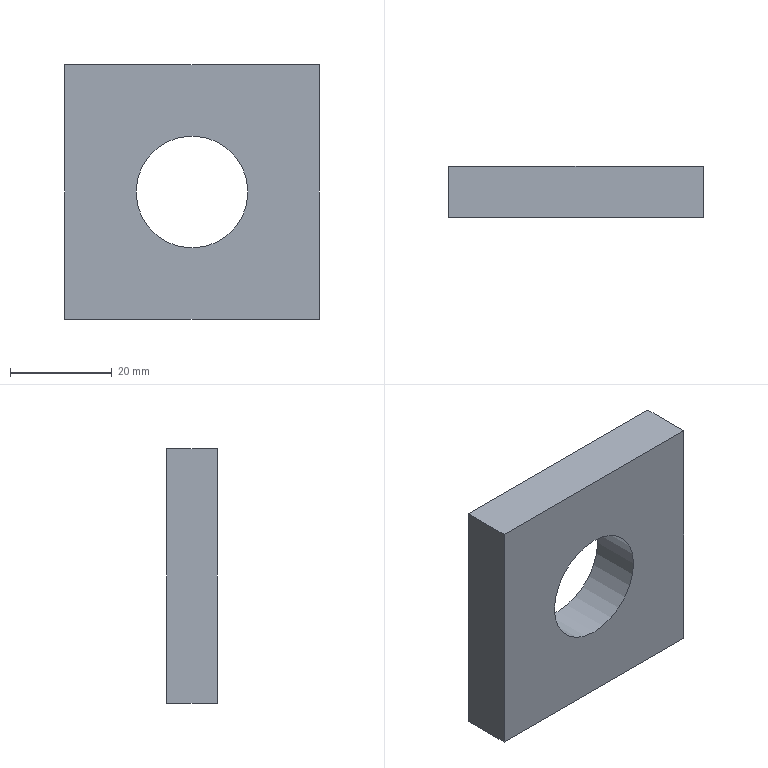Part | STEP file | PN_0016 anchor bolt shim_Default<As Machined> | 1 solid | 7 faces | box 50 x 10 x 50 mm | volume 21199 mm3 | plane 6 | cylinder 1 | commonest cylinder face diameters 22 x1
STEP:
#1=CARTESIAN_POINT('',(0.,0.,0.));
#2=DIRECTION('',(0.,0.,1.));
#3=DIRECTION('',(1.,0.,0.));
#4=AXIS2_PLACEMENT_3D('',#1,#2,#3);
#5=CARTESIAN_POINT('',(25.,10.,25.));
#6=VERTEX_POINT('',#5);
#7=CARTESIAN_POINT('',(25.,10.,-25.));
#8=VERTEX_POINT('',#7);
#9=CARTESIAN_POINT('',(25.,10.,25.));
#10=DIRECTION('',(0.,0.,-1.));
#11=VECTOR('',#10,1.);
#12=LINE('',#9,#11);
#13=CARTESIAN_POINT('',(0.,10.,0.));
#14=DIRECTION('',(0.,-1.,0.));
#15=DIRECTION('',(0.,0.,-1.));
#16=AXIS2_PLACEMENT_3D('',#13,#14,#15);
#17=PLANE('',#16);
#18=CARTESIAN_POINT('',(-25.,25.));
#19=DIRECTION('',(1.,0.));
#20=VECTOR('',#19,1.);
#21=LINE('',#18,#20);
#22=(GEOMETRIC_REPRESENTATION_CONTEXT(2)PARAMETRIC_REPRESENTATION_CONTEXT()REPRESENTATION_CONTEXT('',''));
#23=DEFINITIONAL_REPRESENTATION('',(#21),#22);
#24=PCURVE('',#17,#23);
#25=CARTESIAN_POINT('',(25.,10.,25.));
#26=DIRECTION('',(-1.,0.,0.));
#27=DIRECTION('',(0.,0.,1.));
#28=AXIS2_PLACEMENT_3D('',#25,#26,#27);
#29=PLANE('',#28);
#30=CARTESIAN_POINT('',(0.,0.));
#31=DIRECTION('',(-1.,0.));
#32=VECTOR('',#31,1.);
#33=LINE('',#30,#32);
#34=(GEOMETRIC_REPRESENTATION_CONTEXT(2)PARAMETRIC_REPRESENTATION_CONTEXT()REPRESENTATION_CONTEXT('',''));
#35=DEFINITIONAL_REPRESENTATION('',(#33),#34);
#36=PCURVE('',#29,#35);
#37=SURFACE_CURVE('',#12,(#24,#36),.PCURVE_S1.);
#38=EDGE_CURVE('',#6,#8,#37,.T.);
#39=ORIENTED_EDGE('',*,*,#38,.T.);
#40=CARTESIAN_POINT('',(-25.,10.,-25.));
#41=VERTEX_POINT('',#40);
#42=CARTESIAN_POINT('',(-25.,10.,-25.));
#43=DIRECTION('',(-1.,0.,0.));
#44=VECTOR('',#43,1.);
#45=LINE('',#42,#44);
#46=CARTESIAN_POINT('',(25.,-25.));
#47=DIRECTION('',(0.,-1.));
#48=VECTOR('',#47,1.);
#49=LINE('',#46,#48);
#50=(GEOMETRIC_REPRESENTATION_CONTEXT(2)PARAMETRIC_REPRESENTATION_CONTEXT()REPRESENTATION_CONTEXT('',''));
#51=DEFINITIONAL_REPRESENTATION('',(#49),#50);
#52=PCURVE('',#17,#51);
#53=CARTESIAN_POINT('',(-25.,10.,-25.));
#54=DIRECTION('',(0.,0.,1.));
#55=DIRECTION('',(1.,0.,0.));
#56=AXIS2_PLACEMENT_3D('',#53,#54,#55);
#57=PLANE('',#56);
#58=CARTESIAN_POINT('',(0.,0.));
#59=DIRECTION('',(-1.,0.));
#60=VECTOR('',#59,1.);
#61=LINE('',#58,#60);
#62=(GEOMETRIC_REPRESENTATION_CONTEXT(2)PARAMETRIC_REPRESENTATION_CONTEXT()REPRESENTATION_CONTEXT('',''));
#63=DEFINITIONAL_REPRESENTATION('',(#61),#62);
#64=PCURVE('',#57,#63);
#65=SURFACE_CURVE('',#45,(#52,#64),.PCURVE_S1.);
#66=EDGE_CURVE('',#8,#41,#65,.T.);
#67=ORIENTED_EDGE('',*,*,#66,.T.);
#68=CARTESIAN_POINT('',(-25.,10.,25.));
#69=VERTEX_POINT('',#68);
#70=CARTESIAN_POINT('',(-25.,10.,25.));
#71=DIRECTION('',(0.,0.,1.));
#72=VECTOR('',#71,1.);
#73=LINE('',#70,#72);
#74=CARTESIAN_POINT('',(-25.,-25.));
#75=DIRECTION('',(-1.,0.));
#76=VECTOR('',#75,1.);
#77=LINE('',#74,#76);
#78=(GEOMETRIC_REPRESENTATION_CONTEXT(2)PARAMETRIC_REPRESENTATION_CONTEXT()REPRESENTATION_CONTEXT('',''));
#79=DEFINITIONAL_REPRESENTATION('',(#77),#78);
#80=PCURVE('',#17,#79);
#81=CARTESIAN_POINT('',(-25.,10.,25.));
#82=DIRECTION('',(1.,0.,0.));
#83=DIRECTION('',(0.,0.,-1.));
#84=AXIS2_PLACEMENT_3D('',#81,#82,#83);
#85=PLANE('',#84);
#86=CARTESIAN_POINT('',(0.,0.));
#87=DIRECTION('',(-1.,0.));
#88=VECTOR('',#87,1.);
#89=LINE('',#86,#88);
#90=(GEOMETRIC_REPRESENTATION_CONTEXT(2)PARAMETRIC_REPRESENTATION_CONTEXT()REPRESENTATION_CONTEXT('',''));
#91=DEFINITIONAL_REPRESENTATION('',(#89),#90);
#92=PCURVE('',#85,#91);
#93=SURFACE_CURVE('',#73,(#80,#92),.PCURVE_S1.);
#94=EDGE_CURVE('',#41,#69,#93,.T.);
#95=ORIENTED_EDGE('',*,*,#94,.T.);
#96=CARTESIAN_POINT('',(-25.,10.,25.));
#97=DIRECTION('',(1.,0.,0.));
#98=VECTOR('',#97,1.);
#99=LINE('',#96,#98);
#100=CARTESIAN_POINT('',(-25.,-25.));
#101=DIRECTION('',(0.,1.));
#102=VECTOR('',#101,1.);
#103=LINE('',#100,#102);
#104=(GEOMETRIC_REPRESENTATION_CONTEXT(2)PARAMETRIC_REPRESENTATION_CONTEXT()REPRESENTATION_CONTEXT('',''));
#105=DEFINITIONAL_REPRESENTATION('',(#103),#104);
#106=PCURVE('',#17,#105);
#107=CARTESIAN_POINT('',(-25.,10.,25.));
#108=DIRECTION('',(0.,0.,-1.));
#109=DIRECTION('',(-1.,0.,0.));
#110=AXIS2_PLACEMENT_3D('',#107,#108,#109);
#111=PLANE('',#110);
#112=CARTESIAN_POINT('',(0.,0.));
#113=DIRECTION('',(-1.,0.));
#114=VECTOR('',#113,1.);
#115=LINE('',#112,#114);
#116=(GEOMETRIC_REPRESENTATION_CONTEXT(2)PARAMETRIC_REPRESENTATION_CONTEXT()REPRESENTATION_CONTEXT('',''));
#117=DEFINITIONAL_REPRESENTATION('',(#115),#116);
#118=PCURVE('',#111,#117);
#119=SURFACE_CURVE('',#99,(#106,#118),.PCURVE_S1.);
#120=EDGE_CURVE('',#69,#6,#119,.T.);
#121=ORIENTED_EDGE('',*,*,#120,.T.);
#122=EDGE_LOOP('',(#39,#67,#95,#121));
#123=FACE_BOUND('',#122,.T.);
#124=CARTESIAN_POINT('',(0.,10.,11.));
#125=VERTEX_POINT('',#124);
#126=CARTESIAN_POINT('',(0.,10.,0.));
#127=DIRECTION('',(0.,1.,0.));
#128=DIRECTION('',(0.,0.,1.));
#129=AXIS2_PLACEMENT_3D('',#126,#127,#128);
#130=CIRCLE('',#129,11.);
#131=CARTESIAN_POINT('',(-11.,0.));
#132=CARTESIAN_POINT('',(-11.,19.053));
#133=CARTESIAN_POINT('',(5.5,9.526));
#134=CARTESIAN_POINT('',(22.,0.));
#135=CARTESIAN_POINT('',(5.5,-9.526));
#136=CARTESIAN_POINT('',(-11.,-19.053));
#137=CARTESIAN_POINT('',(-11.,0.));
#138=(BOUNDED_CURVE()B_SPLINE_CURVE(2,(#131,#132,#133,#134,#135,#136,#137),.UNSPECIFIED.,.T.,.F.)B_SPLINE_CURVE_WITH_KNOTS((1,2,2,2,2,1),(-2.094,0.,2.094,4.189,6.283,8.378),.UNSPECIFIED.)CURVE()GEOMETRIC_REPRESENTATION_ITEM()RATIONAL_B_SPLINE_CURVE((1.,0.5,1.,0.5,1.,0.5,1.))REPRESENTATION_ITEM(''));
#139=(GEOMETRIC_REPRESENTATION_CONTEXT(2)PARAMETRIC_REPRESENTATION_CONTEXT()REPRESENTATION_CONTEXT('',''));
#140=DEFINITIONAL_REPRESENTATION('',(#138),#139);
#141=PCURVE('',#17,#140);
#142=CARTESIAN_POINT('',(0.,10.,0.));
#143=DIRECTION('',(0.,-1.,0.));
#144=DIRECTION('',(0.,0.,-1.));
#145=AXIS2_PLACEMENT_3D('',#142,#143,#144);
#146=CYLINDRICAL_SURFACE('',#145,11.);
#147=CARTESIAN_POINT('',(9.425,0.));
#148=DIRECTION('',(-1.,0.));
#149=VECTOR('',#148,1.);
#150=LINE('',#147,#149);
#151=(GEOMETRIC_REPRESENTATION_CONTEXT(2)PARAMETRIC_REPRESENTATION_CONTEXT()REPRESENTATION_CONTEXT('',''));
#152=DEFINITIONAL_REPRESENTATION('',(#150),#151);
#153=PCURVE('',#146,#152);
#154=SURFACE_CURVE('',#130,(#141,#153),.PCURVE_S1.);
#155=EDGE_CURVE('',#125,#125,#154,.T.);
#156=ORIENTED_EDGE('',*,*,#155,.F.);
#157=EDGE_LOOP('',(#156));
#158=FACE_BOUND('',#157,.T.);
#159=ADVANCED_FACE('',(#123,#158),#17,.F.);
#160=CARTESIAN_POINT('',(25.,0.,25.));
#161=VERTEX_POINT('',#160);
#162=CARTESIAN_POINT('',(25.,0.,-25.));
#163=VERTEX_POINT('',#162);
#164=CARTESIAN_POINT('',(25.,0.,25.));
#165=DIRECTION('',(0.,0.,-1.));
#166=VECTOR('',#165,1.);
#167=LINE('',#164,#166);
#168=CARTESIAN_POINT('',(0.,0.,0.));
#169=DIRECTION('',(0.,-1.,0.));
#170=DIRECTION('',(0.,0.,-1.));
#171=AXIS2_PLACEMENT_3D('',#168,#169,#170);
#172=PLANE('',#171);
#173=CARTESIAN_POINT('',(-25.,25.));
#174=DIRECTION('',(1.,0.));
#175=VECTOR('',#174,1.);
#176=LINE('',#173,#175);
#177=(GEOMETRIC_REPRESENTATION_CONTEXT(2)PARAMETRIC_REPRESENTATION_CONTEXT()REPRESENTATION_CONTEXT('',''));
#178=DEFINITIONAL_REPRESENTATION('',(#176),#177);
#179=PCURVE('',#172,#178);
#180=CARTESIAN_POINT('',(0.,-10.));
#181=DIRECTION('',(-1.,0.));
#182=VECTOR('',#181,1.);
#183=LINE('',#180,#182);
#184=(GEOMETRIC_REPRESENTATION_CONTEXT(2)PARAMETRIC_REPRESENTATION_CONTEXT()REPRESENTATION_CONTEXT('',''));
#185=DEFINITIONAL_REPRESENTATION('',(#183),#184);
#186=PCURVE('',#29,#185);
#187=SURFACE_CURVE('',#167,(#179,#186),.PCURVE_S1.);
#188=EDGE_CURVE('',#161,#163,#187,.T.);
#189=ORIENTED_EDGE('',*,*,#188,.F.);
#190=CARTESIAN_POINT('',(-25.,0.,25.));
#191=VERTEX_POINT('',#190);
#192=CARTESIAN_POINT('',(-25.,0.,25.));
#193=DIRECTION('',(1.,0.,0.));
#194=VECTOR('',#193,1.);
#195=LINE('',#192,#194);
#196=CARTESIAN_POINT('',(-25.,-25.));
#197=DIRECTION('',(0.,1.));
#198=VECTOR('',#197,1.);
#199=LINE('',#196,#198);
#200=(GEOMETRIC_REPRESENTATION_CONTEXT(2)PARAMETRIC_REPRESENTATION_CONTEXT()REPRESENTATION_CONTEXT('',''));
#201=DEFINITIONAL_REPRESENTATION('',(#199),#200);
#202=PCURVE('',#172,#201);
#203=CARTESIAN_POINT('',(0.,-10.));
#204=DIRECTION('',(-1.,0.));
#205=VECTOR('',#204,1.);
#206=LINE('',#203,#205);
#207=(GEOMETRIC_REPRESENTATION_CONTEXT(2)PARAMETRIC_REPRESENTATION_CONTEXT()REPRESENTATION_CONTEXT('',''));
#208=DEFINITIONAL_REPRESENTATION('',(#206),#207);
#209=PCURVE('',#111,#208);
#210=SURFACE_CURVE('',#195,(#202,#209),.PCURVE_S1.);
#211=EDGE_CURVE('',#191,#161,#210,.T.);
#212=ORIENTED_EDGE('',*,*,#211,.F.);
#213=CARTESIAN_POINT('',(-25.,0.,-25.));
#214=VERTEX_POINT('',#213);
#215=CARTESIAN_POINT('',(-25.,0.,25.));
#216=DIRECTION('',(0.,0.,1.));
#217=VECTOR('',#216,1.);
#218=LINE('',#215,#217);
#219=CARTESIAN_POINT('',(-25.,-25.));
#220=DIRECTION('',(-1.,0.));
#221=VECTOR('',#220,1.);
#222=LINE('',#219,#221);
#223=(GEOMETRIC_REPRESENTATION_CONTEXT(2)PARAMETRIC_REPRESENTATION_CONTEXT()REPRESENTATION_CONTEXT('',''));
#224=DEFINITIONAL_REPRESENTATION('',(#222),#223);
#225=PCURVE('',#172,#224);
#226=CARTESIAN_POINT('',(0.,-10.));
#227=DIRECTION('',(-1.,0.));
#228=VECTOR('',#227,1.);
#229=LINE('',#226,#228);
#230=(GEOMETRIC_REPRESENTATION_CONTEXT(2)PARAMETRIC_REPRESENTATION_CONTEXT()REPRESENTATION_CONTEXT('',''));
#231=DEFINITIONAL_REPRESENTATION('',(#229),#230);
#232=PCURVE('',#85,#231);
#233=SURFACE_CURVE('',#218,(#225,#232),.PCURVE_S1.);
#234=EDGE_CURVE('',#214,#191,#233,.T.);
#235=ORIENTED_EDGE('',*,*,#234,.F.);
#236=CARTESIAN_POINT('',(-25.,0.,-25.));
#237=DIRECTION('',(-1.,0.,0.));
#238=VECTOR('',#237,1.);
#239=LINE('',#236,#238);
#240=CARTESIAN_POINT('',(25.,-25.));
#241=DIRECTION('',(0.,-1.));
#242=VECTOR('',#241,1.);
#243=LINE('',#240,#242);
#244=(GEOMETRIC_REPRESENTATION_CONTEXT(2)PARAMETRIC_REPRESENTATION_CONTEXT()REPRESENTATION_CONTEXT('',''));
#245=DEFINITIONAL_REPRESENTATION('',(#243),#244);
#246=PCURVE('',#172,#245);
#247=CARTESIAN_POINT('',(0.,-10.));
#248=DIRECTION('',(-1.,0.));
#249=VECTOR('',#248,1.);
#250=LINE('',#247,#249);
#251=(GEOMETRIC_REPRESENTATION_CONTEXT(2)PARAMETRIC_REPRESENTATION_CONTEXT()REPRESENTATION_CONTEXT('',''));
#252=DEFINITIONAL_REPRESENTATION('',(#250),#251);
#253=PCURVE('',#57,#252);
#254=SURFACE_CURVE('',#239,(#246,#253),.PCURVE_S1.);
#255=EDGE_CURVE('',#163,#214,#254,.T.);
#256=ORIENTED_EDGE('',*,*,#255,.F.);
#257=EDGE_LOOP('',(#189,#212,#235,#256));
#258=FACE_BOUND('',#257,.T.);
#259=CARTESIAN_POINT('',(0.,0.,11.));
#260=VERTEX_POINT('',#259);
#261=CARTESIAN_POINT('',(0.,0.,0.));
#262=DIRECTION('',(0.,1.,0.));
#263=DIRECTION('',(0.,0.,1.));
#264=AXIS2_PLACEMENT_3D('',#261,#262,#263);
#265=CIRCLE('',#264,11.);
#266=CARTESIAN_POINT('',(-11.,0.));
#267=CARTESIAN_POINT('',(-11.,19.053));
#268=CARTESIAN_POINT('',(5.5,9.526));
#269=CARTESIAN_POINT('',(22.,0.));
#270=CARTESIAN_POINT('',(5.5,-9.526));
#271=CARTESIAN_POINT('',(-11.,-19.053));
#272=CARTESIAN_POINT('',(-11.,0.));
#273=(BOUNDED_CURVE()B_SPLINE_CURVE(2,(#266,#267,#268,#269,#270,#271,#272),.UNSPECIFIED.,.T.,.F.)B_SPLINE_CURVE_WITH_KNOTS((1,2,2,2,2,1),(-2.094,0.,2.094,4.189,6.283,8.378),.UNSPECIFIED.)CURVE()GEOMETRIC_REPRESENTATION_ITEM()RATIONAL_B_SPLINE_CURVE((1.,0.5,1.,0.5,1.,0.5,1.))REPRESENTATION_ITEM(''));
#274=(GEOMETRIC_REPRESENTATION_CONTEXT(2)PARAMETRIC_REPRESENTATION_CONTEXT()REPRESENTATION_CONTEXT('',''));
#275=DEFINITIONAL_REPRESENTATION('',(#273),#274);
#276=PCURVE('',#172,#275);
#277=CARTESIAN_POINT('',(9.425,10.));
#278=DIRECTION('',(-1.,0.));
#279=VECTOR('',#278,1.);
#280=LINE('',#277,#279);
#281=(GEOMETRIC_REPRESENTATION_CONTEXT(2)PARAMETRIC_REPRESENTATION_CONTEXT()REPRESENTATION_CONTEXT('',''));
#282=DEFINITIONAL_REPRESENTATION('',(#280),#281);
#283=PCURVE('',#146,#282);
#284=SURFACE_CURVE('',#265,(#276,#283),.PCURVE_S1.);
#285=EDGE_CURVE('',#260,#260,#284,.T.);
#286=ORIENTED_EDGE('',*,*,#285,.T.);
#287=EDGE_LOOP('',(#286));
#288=FACE_BOUND('',#287,.T.);
#289=ADVANCED_FACE('',(#258,#288),#172,.T.);
#290=ORIENTED_EDGE('',*,*,#188,.T.);
#291=CARTESIAN_POINT('',(25.,10.,-25.));
#292=DIRECTION('',(0.,-1.,0.));
#293=VECTOR('',#292,1.);
#294=LINE('',#291,#293);
#295=CARTESIAN_POINT('',(-50.,0.));
#296=DIRECTION('',(0.,-1.));
#297=VECTOR('',#296,1.);
#298=LINE('',#295,#297);
#299=(GEOMETRIC_REPRESENTATION_CONTEXT(2)PARAMETRIC_REPRESENTATION_CONTEXT()REPRESENTATION_CONTEXT('',''));
#300=DEFINITIONAL_REPRESENTATION('',(#298),#299);
#301=PCURVE('',#29,#300);
#302=CARTESIAN_POINT('',(50.,0.));
#303=DIRECTION('',(0.,-1.));
#304=VECTOR('',#303,1.);
#305=LINE('',#302,#304);
#306=(GEOMETRIC_REPRESENTATION_CONTEXT(2)PARAMETRIC_REPRESENTATION_CONTEXT()REPRESENTATION_CONTEXT('',''));
#307=DEFINITIONAL_REPRESENTATION('',(#305),#306);
#308=PCURVE('',#57,#307);
#309=SURFACE_CURVE('',#294,(#301,#308),.PCURVE_S1.);
#310=EDGE_CURVE('',#8,#163,#309,.T.);
#311=ORIENTED_EDGE('',*,*,#310,.F.);
#312=ORIENTED_EDGE('',*,*,#38,.F.);
#313=CARTESIAN_POINT('',(25.,10.,25.));
#314=DIRECTION('',(0.,-1.,0.));
#315=VECTOR('',#314,1.);
#316=LINE('',#313,#315);
#317=CARTESIAN_POINT('',(0.,0.));
#318=DIRECTION('',(0.,-1.));
#319=VECTOR('',#318,1.);
#320=LINE('',#317,#319);
#321=(GEOMETRIC_REPRESENTATION_CONTEXT(2)PARAMETRIC_REPRESENTATION_CONTEXT()REPRESENTATION_CONTEXT('',''));
#322=DEFINITIONAL_REPRESENTATION('',(#320),#321);
#323=PCURVE('',#29,#322);
#324=CARTESIAN_POINT('',(-50.,0.));
#325=DIRECTION('',(0.,-1.));
#326=VECTOR('',#325,1.);
#327=LINE('',#324,#326);
#328=(GEOMETRIC_REPRESENTATION_CONTEXT(2)PARAMETRIC_REPRESENTATION_CONTEXT()REPRESENTATION_CONTEXT('',''));
#329=DEFINITIONAL_REPRESENTATION('',(#327),#328);
#330=PCURVE('',#111,#329);
#331=SURFACE_CURVE('',#316,(#323,#330),.PCURVE_S1.);
#332=EDGE_CURVE('',#6,#161,#331,.T.);
#333=ORIENTED_EDGE('',*,*,#332,.T.);
#334=EDGE_LOOP('',(#290,#311,#312,#333));
#335=FACE_BOUND('',#334,.T.);
#336=ADVANCED_FACE('',(#335),#29,.F.);
#337=ORIENTED_EDGE('',*,*,#255,.T.);
#338=CARTESIAN_POINT('',(-25.,10.,-25.));
#339=DIRECTION('',(0.,-1.,0.));
#340=VECTOR('',#339,1.);
#341=LINE('',#338,#340);
#342=CARTESIAN_POINT('',(0.,0.));
#343=DIRECTION('',(0.,-1.));
#344=VECTOR('',#343,1.);
#345=LINE('',#342,#344);
#346=(GEOMETRIC_REPRESENTATION_CONTEXT(2)PARAMETRIC_REPRESENTATION_CONTEXT()REPRESENTATION_CONTEXT('',''));
#347=DEFINITIONAL_REPRESENTATION('',(#345),#346);
#348=PCURVE('',#57,#347);
#349=CARTESIAN_POINT('',(50.,0.));
#350=DIRECTION('',(0.,-1.));
#351=VECTOR('',#350,1.);
#352=LINE('',#349,#351);
#353=(GEOMETRIC_REPRESENTATION_CONTEXT(2)PARAMETRIC_REPRESENTATION_CONTEXT()REPRESENTATION_CONTEXT('',''));
#354=DEFINITIONAL_REPRESENTATION('',(#352),#353);
#355=PCURVE('',#85,#354);
#356=SURFACE_CURVE('',#341,(#348,#355),.PCURVE_S1.);
#357=EDGE_CURVE('',#41,#214,#356,.T.);
#358=ORIENTED_EDGE('',*,*,#357,.F.);
#359=ORIENTED_EDGE('',*,*,#66,.F.);
#360=ORIENTED_EDGE('',*,*,#310,.T.);
#361=EDGE_LOOP('',(#337,#358,#359,#360));
#362=FACE_BOUND('',#361,.T.);
#363=ADVANCED_FACE('',(#362),#57,.F.);
#364=ORIENTED_EDGE('',*,*,#234,.T.);
#365=CARTESIAN_POINT('',(-25.,10.,25.));
#366=DIRECTION('',(0.,-1.,0.));
#367=VECTOR('',#366,1.);
#368=LINE('',#365,#367);
#369=CARTESIAN_POINT('',(0.,0.));
#370=DIRECTION('',(0.,-1.));
#371=VECTOR('',#370,1.);
#372=LINE('',#369,#371);
#373=(GEOMETRIC_REPRESENTATION_CONTEXT(2)PARAMETRIC_REPRESENTATION_CONTEXT()REPRESENTATION_CONTEXT('',''));
#374=DEFINITIONAL_REPRESENTATION('',(#372),#373);
#375=PCURVE('',#85,#374);
#376=CARTESIAN_POINT('',(0.,0.));
#377=DIRECTION('',(0.,-1.));
#378=VECTOR('',#377,1.);
#379=LINE('',#376,#378);
#380=(GEOMETRIC_REPRESENTATION_CONTEXT(2)PARAMETRIC_REPRESENTATION_CONTEXT()REPRESENTATION_CONTEXT('',''));
#381=DEFINITIONAL_REPRESENTATION('',(#379),#380);
#382=PCURVE('',#111,#381);
#383=SURFACE_CURVE('',#368,(#375,#382),.PCURVE_S1.);
#384=EDGE_CURVE('',#69,#191,#383,.T.);
#385=ORIENTED_EDGE('',*,*,#384,.F.);
#386=ORIENTED_EDGE('',*,*,#94,.F.);
#387=ORIENTED_EDGE('',*,*,#357,.T.);
#388=EDGE_LOOP('',(#364,#385,#386,#387));
#389=FACE_BOUND('',#388,.T.);
#390=ADVANCED_FACE('',(#389),#85,.F.);
#391=ORIENTED_EDGE('',*,*,#211,.T.);
#392=ORIENTED_EDGE('',*,*,#332,.F.);
#393=ORIENTED_EDGE('',*,*,#120,.F.);
#394=ORIENTED_EDGE('',*,*,#384,.T.);
#395=EDGE_LOOP('',(#391,#392,#393,#394));
#396=FACE_BOUND('',#395,.T.);
#397=ADVANCED_FACE('',(#396),#111,.F.);
#398=ORIENTED_EDGE('',*,*,#155,.F.);
#399=CARTESIAN_POINT('',(0.,10.,11.));
#400=CARTESIAN_POINT('',(0.,0.,11.));
#401=B_SPLINE_CURVE_WITH_KNOTS('',1,(#399,#400),.UNSPECIFIED.,.F.,.F.,(2,2),(0.,10.),.PIECEWISE_BEZIER_KNOTS.);
#402=CARTESIAN_POINT('',(9.425,0.));
#403=DIRECTION('',(0.,1.));
#404=VECTOR('',#403,1.);
#405=LINE('',#402,#404);
#406=(GEOMETRIC_REPRESENTATION_CONTEXT(2)PARAMETRIC_REPRESENTATION_CONTEXT()REPRESENTATION_CONTEXT('',''));
#407=DEFINITIONAL_REPRESENTATION('',(#405),#406);
#408=PCURVE('',#146,#407);
#409=CARTESIAN_POINT('',(3.142,0.));
#410=DIRECTION('',(0.,1.));
#411=VECTOR('',#410,1.);
#412=LINE('',#409,#411);
#413=(GEOMETRIC_REPRESENTATION_CONTEXT(2)PARAMETRIC_REPRESENTATION_CONTEXT()REPRESENTATION_CONTEXT('',''));
#414=DEFINITIONAL_REPRESENTATION('',(#412),#413);
#415=PCURVE('',#146,#414);
#416=SEAM_CURVE('',#401,(#408,#415),.PCURVE_S1.);
#417=EDGE_CURVE('',#125,#260,#416,.T.);
#418=ORIENTED_EDGE('',*,*,#417,.T.);
#419=ORIENTED_EDGE('',*,*,#285,.T.);
#420=ORIENTED_EDGE('',*,*,#417,.F.);
#421=EDGE_LOOP('',(#398,#418,#419,#420));
#422=FACE_BOUND('',#421,.F.);
#423=ADVANCED_FACE('',(#422),#146,.F.);
#424=CLOSED_SHELL('',(#159,#289,#336,#363,#390,#397,#423));
#425=MANIFOLD_SOLID_BREP('',#424);
#426=(LENGTH_UNIT()NAMED_UNIT(*)SI_UNIT(.MILLI.,.METRE.));
#427=UNCERTAINTY_MEASURE_WITH_UNIT(LENGTH_MEASURE(0.000002),#426,'','');
#428=(NAMED_UNIT(*)PLANE_ANGLE_UNIT()SI_UNIT($,.RADIAN.));
#429=(NAMED_UNIT(*)SI_UNIT($,.STERADIAN.)SOLID_ANGLE_UNIT());
#430=(GEOMETRIC_REPRESENTATION_CONTEXT(3)GLOBAL_UNCERTAINTY_ASSIGNED_CONTEXT((#427))GLOBAL_UNIT_ASSIGNED_CONTEXT((#426,#428,#429))REPRESENTATION_CONTEXT('',''));
#431=ADVANCED_BREP_SHAPE_REPRESENTATION('',(#4,#425),#430);